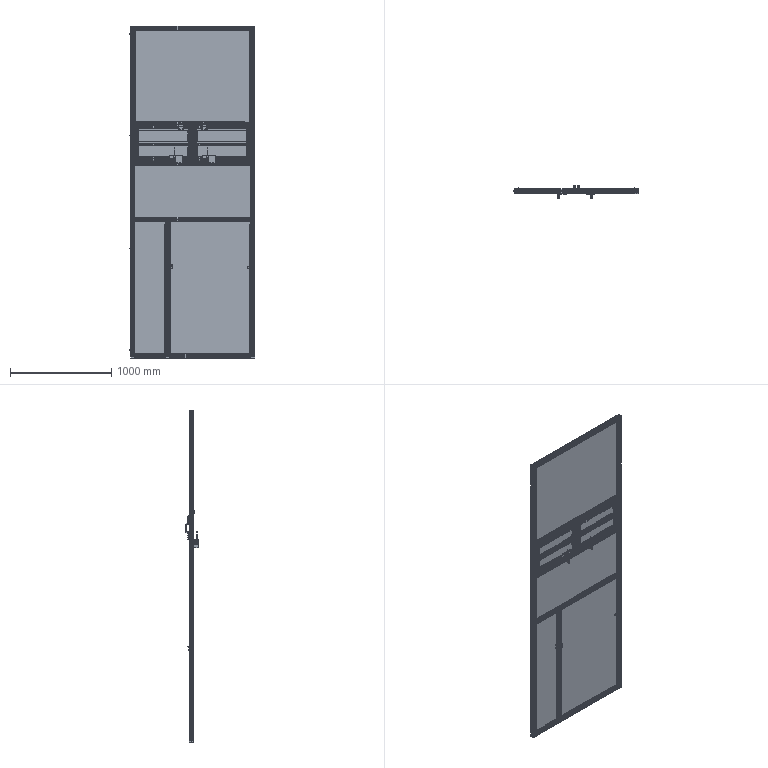Part | SolidWorks | features ReferencePattern 79, LocalLPattern 15, MirrorCompFeat 6, CompositeCurve 2 | 217 solids | 12196 faces | volume 27416958 mm3 | plane 7938 | cylinder 2614 | cone 828 | spline 748 | torus 48 | sphere 20 | commonest cylinder face diameters 6.8 x330 2 x264 19 x168 5 x148 1.5 x132 0.562 x110